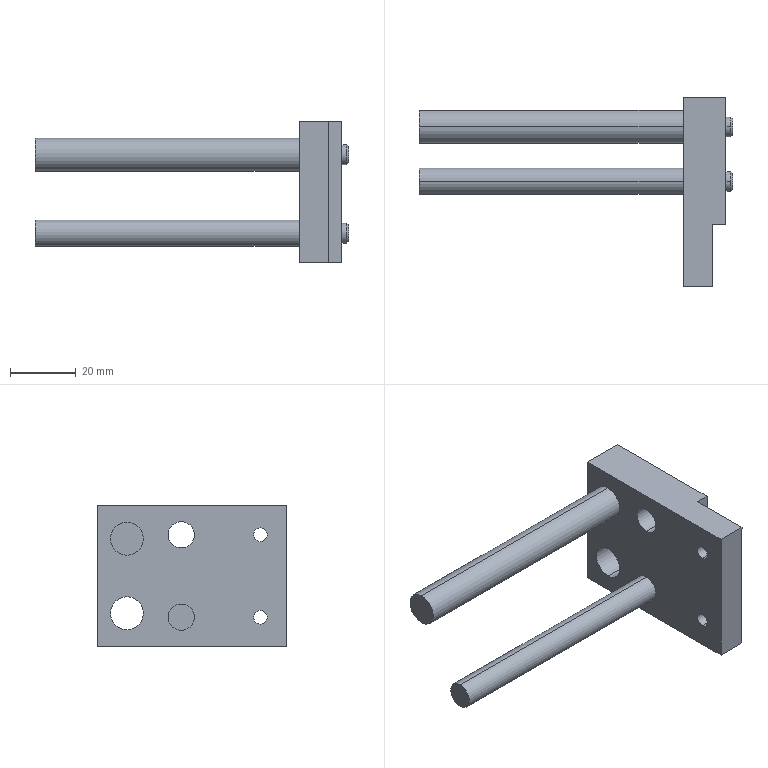Part | SolidWorks | features BaseBody 1 | 1 solid | 58 faces | box 95 x 57.5 x 43 mm | volume 36178 mm3 | cylinder 28 | plane 18 | cone 8 | torus 4 | commonest cylinder face diameters 10 x8 4.134 x4 6 x4 8 x4 12.5 x4 15 x4